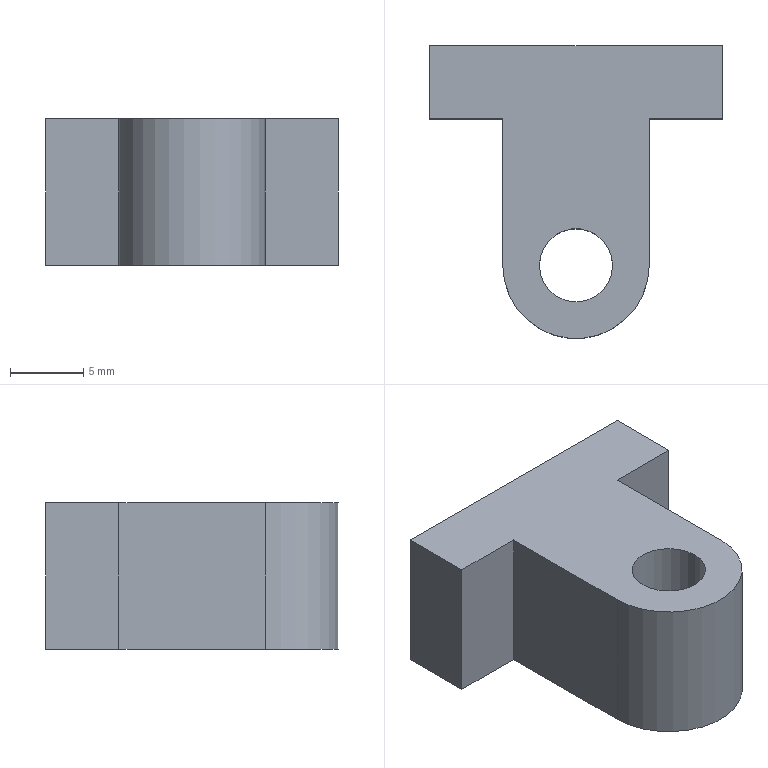Part | SolidWorks | features Extrusion 1, ICE 1 | 1 solid | 15 faces | box 20 x 20 x 10 mm | volume 2177 mm3 | plane 10 | cylinder 5 | commonest cylinder face diameters 5 x4 10 x1
STEP:
#1=CARTESIAN_POINT('',(0.,14.,2.5));
#2=VERTEX_POINT('',#1);
#3=CARTESIAN_POINT('',(0.,14.,7.5));
#4=VERTEX_POINT('',#3);
#5=CARTESIAN_POINT('',(0.,14.,5.));
#6=DIRECTION('',(0.,1.,0.));
#7=DIRECTION('',(0.,0.,1.));
#8=AXIS2_PLACEMENT_3D('',#5,#6,#7);
#9=CIRCLE('',#8,2.5);
#10=EDGE_CURVE('',#2,#4,#9,.T.);
#11=ORIENTED_EDGE('',*,*,#10,.F.);
#12=CARTESIAN_POINT('',(0.,15.,2.5));
#13=VERTEX_POINT('',#12);
#14=CARTESIAN_POINT('',(0.,14.,2.5));
#15=DIRECTION('',(0.,1.,0.));
#16=VECTOR('',#15,1000.);
#17=LINE('',#14,#16);
#18=EDGE_CURVE('',#2,#13,#17,.T.);
#19=ORIENTED_EDGE('',*,*,#18,.T.);
#20=CARTESIAN_POINT('',(0.,15.,7.5));
#21=VERTEX_POINT('',#20);
#22=CARTESIAN_POINT('',(0.,15.,5.));
#23=DIRECTION('',(0.,1.,0.));
#24=DIRECTION('',(0.,0.,1.));
#25=AXIS2_PLACEMENT_3D('',#22,#23,#24);
#26=CIRCLE('',#25,2.5);
#27=EDGE_CURVE('',#13,#21,#26,.T.);
#28=ORIENTED_EDGE('',*,*,#27,.T.);
#29=CARTESIAN_POINT('',(0.,14.,7.5));
#30=DIRECTION('',(0.,1.,0.));
#31=VECTOR('',#30,1000.);
#32=LINE('',#29,#31);
#33=EDGE_CURVE('',#4,#21,#32,.T.);
#34=ORIENTED_EDGE('',*,*,#33,.F.);
#35=EDGE_LOOP('',(#11,#19,#28,#34));
#36=FACE_OUTER_BOUND('',#35,.T.);
#37=CARTESIAN_POINT('',(0.,14.,5.));
#38=DIRECTION('',(0.,1.,0.));
#39=DIRECTION('',(0.,0.,1.));
#40=AXIS2_PLACEMENT_3D('',#37,#38,#39);
#41=CYLINDRICAL_SURFACE('',#40,2.5);
#42=ADVANCED_FACE('',(#36),#41,.F.);
#43=CARTESIAN_POINT('',(-2.5,0.,10.));
#44=VERTEX_POINT('',#43);
#45=CARTESIAN_POINT('',(2.5,0.,10.));
#46=VERTEX_POINT('',#45);
#47=CARTESIAN_POINT('',(0.,0.,10.));
#48=DIRECTION('',(0.,0.,1.));
#49=DIRECTION('',(1.,0.,0.));
#50=AXIS2_PLACEMENT_3D('',#47,#48,#49);
#51=CIRCLE('',#50,2.5);
#52=EDGE_CURVE('',#44,#46,#51,.T.);
#53=ORIENTED_EDGE('',*,*,#52,.T.);
#54=CARTESIAN_POINT('',(2.5,0.,0.));
#55=VERTEX_POINT('',#54);
#56=CARTESIAN_POINT('',(2.5,0.,10.));
#57=DIRECTION('',(0.,0.,-1.));
#58=VECTOR('',#57,1000.);
#59=LINE('',#56,#58);
#60=EDGE_CURVE('',#46,#55,#59,.T.);
#61=ORIENTED_EDGE('',*,*,#60,.T.);
#62=CARTESIAN_POINT('',(-2.5,0.,0.));
#63=VERTEX_POINT('',#62);
#64=CARTESIAN_POINT('',(0.,0.,0.));
#65=DIRECTION('',(0.,0.,1.));
#66=DIRECTION('',(1.,0.,0.));
#67=AXIS2_PLACEMENT_3D('',#64,#65,#66);
#68=CIRCLE('',#67,2.5);
#69=EDGE_CURVE('',#63,#55,#68,.T.);
#70=ORIENTED_EDGE('',*,*,#69,.F.);
#71=CARTESIAN_POINT('',(-2.5,0.,10.));
#72=DIRECTION('',(0.,0.,-1.));
#73=VECTOR('',#72,1000.);
#74=LINE('',#71,#73);
#75=EDGE_CURVE('',#44,#63,#74,.T.);
#76=ORIENTED_EDGE('',*,*,#75,.F.);
#77=EDGE_LOOP('',(#53,#61,#70,#76));
#78=FACE_OUTER_BOUND('',#77,.T.);
#79=CARTESIAN_POINT('',(0.,0.,10.));
#80=DIRECTION('',(0.,0.,-1.));
#81=DIRECTION('',(-1.,0.,0.));
#82=AXIS2_PLACEMENT_3D('',#79,#80,#81);
#83=CYLINDRICAL_SURFACE('',#82,2.5);
#84=ADVANCED_FACE('',(#78),#83,.F.);
#85=CARTESIAN_POINT('',(-5.,0.,10.));
#86=VERTEX_POINT('',#85);
#87=CARTESIAN_POINT('',(5.,0.,10.));
#88=VERTEX_POINT('',#87);
#89=CARTESIAN_POINT('',(0.,0.,10.));
#90=DIRECTION('',(0.,0.,1.));
#91=DIRECTION('',(1.,0.,0.));
#92=AXIS2_PLACEMENT_3D('',#89,#90,#91);
#93=CIRCLE('',#92,5.);
#94=EDGE_CURVE('',#86,#88,#93,.T.);
#95=ORIENTED_EDGE('',*,*,#94,.T.);
#96=CARTESIAN_POINT('',(5.,10.,10.));
#97=VERTEX_POINT('',#96);
#98=CARTESIAN_POINT('',(5.,0.,10.));
#99=DIRECTION('',(0.,1.,0.));
#100=VECTOR('',#99,1000.);
#101=LINE('',#98,#100);
#102=EDGE_CURVE('',#88,#97,#101,.T.);
#103=ORIENTED_EDGE('',*,*,#102,.T.);
#104=CARTESIAN_POINT('',(10.,10.,10.));
#105=VERTEX_POINT('',#104);
#106=CARTESIAN_POINT('',(5.,10.,10.));
#107=DIRECTION('',(1.,0.,0.));
#108=VECTOR('',#107,1000.);
#109=LINE('',#106,#108);
#110=EDGE_CURVE('',#97,#105,#109,.T.);
#111=ORIENTED_EDGE('',*,*,#110,.T.);
#112=CARTESIAN_POINT('',(10.,15.,10.));
#113=VERTEX_POINT('',#112);
#114=CARTESIAN_POINT('',(10.,10.,10.));
#115=DIRECTION('',(0.,1.,0.));
#116=VECTOR('',#115,1000.);
#117=LINE('',#114,#116);
#118=EDGE_CURVE('',#105,#113,#117,.T.);
#119=ORIENTED_EDGE('',*,*,#118,.T.);
#120=CARTESIAN_POINT('',(-10.,15.,10.));
#121=VERTEX_POINT('',#120);
#122=CARTESIAN_POINT('',(-10.,15.,10.));
#123=DIRECTION('',(-1.,0.,0.));
#124=VECTOR('',#123,1000.);
#125=LINE('',#122,#124);
#126=EDGE_CURVE('',#113,#121,#125,.T.);
#127=ORIENTED_EDGE('',*,*,#126,.T.);
#128=CARTESIAN_POINT('',(-10.,10.,10.));
#129=VERTEX_POINT('',#128);
#130=CARTESIAN_POINT('',(-10.,10.,10.));
#131=DIRECTION('',(0.,-1.,0.));
#132=VECTOR('',#131,1000.);
#133=LINE('',#130,#132);
#134=EDGE_CURVE('',#121,#129,#133,.T.);
#135=ORIENTED_EDGE('',*,*,#134,.T.);
#136=CARTESIAN_POINT('',(-5.,10.,10.));
#137=VERTEX_POINT('',#136);
#138=CARTESIAN_POINT('',(-5.,10.,10.));
#139=DIRECTION('',(1.,0.,0.));
#140=VECTOR('',#139,1000.);
#141=LINE('',#138,#140);
#142=EDGE_CURVE('',#129,#137,#141,.T.);
#143=ORIENTED_EDGE('',*,*,#142,.T.);
#144=CARTESIAN_POINT('',(-5.,0.,10.));
#145=DIRECTION('',(0.,-1.,0.));
#146=VECTOR('',#145,1000.);
#147=LINE('',#144,#146);
#148=EDGE_CURVE('',#137,#86,#147,.T.);
#149=ORIENTED_EDGE('',*,*,#148,.T.);
#150=EDGE_LOOP('',(#95,#103,#111,#119,#127,#135,#143,#149));
#151=FACE_OUTER_BOUND('',#150,.T.);
#152=ORIENTED_EDGE('',*,*,#52,.F.);
#153=CARTESIAN_POINT('',(0.,0.,10.));
#154=DIRECTION('',(0.,0.,1.));
#155=DIRECTION('',(1.,0.,0.));
#156=AXIS2_PLACEMENT_3D('',#153,#154,#155);
#157=CIRCLE('',#156,2.5);
#158=EDGE_CURVE('',#46,#44,#157,.T.);
#159=ORIENTED_EDGE('',*,*,#158,.F.);
#160=EDGE_LOOP('',(#152,#159));
#161=FACE_BOUND('',#160,.T.);
#162=CARTESIAN_POINT('',(0.,0.,10.));
#163=DIRECTION('',(0.,0.,1.));
#164=DIRECTION('',(1.,0.,0.));
#165=AXIS2_PLACEMENT_3D('',#162,#163,#164);
#166=PLANE('',#165);
#167=ADVANCED_FACE('',(#151,#161),#166,.T.);
#168=CARTESIAN_POINT('',(-5.,0.,0.));
#169=VERTEX_POINT('',#168);
#170=CARTESIAN_POINT('',(5.,0.,0.));
#171=VERTEX_POINT('',#170);
#172=CARTESIAN_POINT('',(0.,0.,0.));
#173=DIRECTION('',(0.,0.,1.));
#174=DIRECTION('',(1.,0.,0.));
#175=AXIS2_PLACEMENT_3D('',#172,#173,#174);
#176=CIRCLE('',#175,5.);
#177=EDGE_CURVE('',#169,#171,#176,.T.);
#178=ORIENTED_EDGE('',*,*,#177,.F.);
#179=CARTESIAN_POINT('',(-5.,10.,0.));
#180=VERTEX_POINT('',#179);
#181=CARTESIAN_POINT('',(-5.,0.,0.));
#182=DIRECTION('',(0.,-1.,0.));
#183=VECTOR('',#182,1000.);
#184=LINE('',#181,#183);
#185=EDGE_CURVE('',#180,#169,#184,.T.);
#186=ORIENTED_EDGE('',*,*,#185,.F.);
#187=CARTESIAN_POINT('',(-10.,10.,0.));
#188=VERTEX_POINT('',#187);
#189=CARTESIAN_POINT('',(-5.,10.,0.));
#190=DIRECTION('',(1.,0.,0.));
#191=VECTOR('',#190,1000.);
#192=LINE('',#189,#191);
#193=EDGE_CURVE('',#188,#180,#192,.T.);
#194=ORIENTED_EDGE('',*,*,#193,.F.);
#195=CARTESIAN_POINT('',(-10.,15.,0.));
#196=VERTEX_POINT('',#195);
#197=CARTESIAN_POINT('',(-10.,10.,0.));
#198=DIRECTION('',(0.,-1.,0.));
#199=VECTOR('',#198,1000.);
#200=LINE('',#197,#199);
#201=EDGE_CURVE('',#196,#188,#200,.T.);
#202=ORIENTED_EDGE('',*,*,#201,.F.);
#203=CARTESIAN_POINT('',(10.,15.,0.));
#204=VERTEX_POINT('',#203);
#205=CARTESIAN_POINT('',(-10.,15.,0.));
#206=DIRECTION('',(-1.,0.,0.));
#207=VECTOR('',#206,1000.);
#208=LINE('',#205,#207);
#209=EDGE_CURVE('',#204,#196,#208,.T.);
#210=ORIENTED_EDGE('',*,*,#209,.F.);
#211=CARTESIAN_POINT('',(10.,10.,0.));
#212=VERTEX_POINT('',#211);
#213=CARTESIAN_POINT('',(10.,10.,0.));
#214=DIRECTION('',(0.,1.,0.));
#215=VECTOR('',#214,1000.);
#216=LINE('',#213,#215);
#217=EDGE_CURVE('',#212,#204,#216,.T.);
#218=ORIENTED_EDGE('',*,*,#217,.F.);
#219=CARTESIAN_POINT('',(5.,10.,0.));
#220=VERTEX_POINT('',#219);
#221=CARTESIAN_POINT('',(5.,10.,0.));
#222=DIRECTION('',(1.,0.,0.));
#223=VECTOR('',#222,1000.);
#224=LINE('',#221,#223);
#225=EDGE_CURVE('',#220,#212,#224,.T.);
#226=ORIENTED_EDGE('',*,*,#225,.F.);
#227=CARTESIAN_POINT('',(5.,0.,0.));
#228=DIRECTION('',(0.,1.,0.));
#229=VECTOR('',#228,1000.);
#230=LINE('',#227,#229);
#231=EDGE_CURVE('',#171,#220,#230,.T.);
#232=ORIENTED_EDGE('',*,*,#231,.F.);
#233=EDGE_LOOP('',(#178,#186,#194,#202,#210,#218,#226,#232));
#234=FACE_OUTER_BOUND('',#233,.T.);
#235=ORIENTED_EDGE('',*,*,#69,.T.);
#236=CARTESIAN_POINT('',(0.,0.,0.));
#237=DIRECTION('',(0.,0.,1.));
#238=DIRECTION('',(1.,0.,0.));
#239=AXIS2_PLACEMENT_3D('',#236,#237,#238);
#240=CIRCLE('',#239,2.5);
#241=EDGE_CURVE('',#55,#63,#240,.T.);
#242=ORIENTED_EDGE('',*,*,#241,.T.);
#243=EDGE_LOOP('',(#235,#242));
#244=FACE_BOUND('',#243,.T.);
#245=CARTESIAN_POINT('',(0.,0.,0.));
#246=DIRECTION('',(0.,0.,1.));
#247=DIRECTION('',(1.,0.,0.));
#248=AXIS2_PLACEMENT_3D('',#245,#246,#247);
#249=PLANE('',#248);
#250=ADVANCED_FACE('',(#234,#244),#249,.F.);
#251=ORIENTED_EDGE('',*,*,#177,.T.);
#252=CARTESIAN_POINT('',(5.,0.,10.));
#253=DIRECTION('',(0.,0.,-1.));
#254=VECTOR('',#253,1000.);
#255=LINE('',#252,#254);
#256=EDGE_CURVE('',#88,#171,#255,.T.);
#257=ORIENTED_EDGE('',*,*,#256,.F.);
#258=ORIENTED_EDGE('',*,*,#94,.F.);
#259=CARTESIAN_POINT('',(-5.,0.,10.));
#260=DIRECTION('',(0.,0.,-1.));
#261=VECTOR('',#260,1000.);
#262=LINE('',#259,#261);
#263=EDGE_CURVE('',#86,#169,#262,.T.);
#264=ORIENTED_EDGE('',*,*,#263,.T.);
#265=EDGE_LOOP('',(#251,#257,#258,#264));
#266=FACE_OUTER_BOUND('',#265,.T.);
#267=CARTESIAN_POINT('',(0.,0.,10.));
#268=DIRECTION('',(0.,0.,-1.));
#269=DIRECTION('',(-1.,0.,0.));
#270=AXIS2_PLACEMENT_3D('',#267,#268,#269);
#271=CYLINDRICAL_SURFACE('',#270,5.);
#272=ADVANCED_FACE('',(#266),#271,.T.);
#273=ORIENTED_EDGE('',*,*,#231,.T.);
#274=CARTESIAN_POINT('',(5.,10.,10.));
#275=DIRECTION('',(0.,0.,-1.));
#276=VECTOR('',#275,1000.);
#277=LINE('',#274,#276);
#278=EDGE_CURVE('',#97,#220,#277,.T.);
#279=ORIENTED_EDGE('',*,*,#278,.F.);
#280=ORIENTED_EDGE('',*,*,#102,.F.);
#281=ORIENTED_EDGE('',*,*,#256,.T.);
#282=EDGE_LOOP('',(#273,#279,#280,#281));
#283=FACE_OUTER_BOUND('',#282,.T.);
#284=CARTESIAN_POINT('',(5.,0.,10.));
#285=DIRECTION('',(-1.,0.,0.));
#286=DIRECTION('',(0.,0.,1.));
#287=AXIS2_PLACEMENT_3D('',#284,#285,#286);
#288=PLANE('',#287);
#289=ADVANCED_FACE('',(#283),#288,.F.);
#290=ORIENTED_EDGE('',*,*,#225,.T.);
#291=CARTESIAN_POINT('',(10.,10.,10.));
#292=DIRECTION('',(0.,0.,-1.));
#293=VECTOR('',#292,1000.);
#294=LINE('',#291,#293);
#295=EDGE_CURVE('',#105,#212,#294,.T.);
#296=ORIENTED_EDGE('',*,*,#295,.F.);
#297=ORIENTED_EDGE('',*,*,#110,.F.);
#298=ORIENTED_EDGE('',*,*,#278,.T.);
#299=EDGE_LOOP('',(#290,#296,#297,#298));
#300=FACE_OUTER_BOUND('',#299,.T.);
#301=CARTESIAN_POINT('',(5.,10.,10.));
#302=DIRECTION('',(0.,1.,0.));
#303=DIRECTION('',(0.,0.,1.));
#304=AXIS2_PLACEMENT_3D('',#301,#302,#303);
#305=PLANE('',#304);
#306=ADVANCED_FACE('',(#300),#305,.F.);
#307=ORIENTED_EDGE('',*,*,#217,.T.);
#308=CARTESIAN_POINT('',(10.,15.,10.));
#309=DIRECTION('',(0.,0.,-1.));
#310=VECTOR('',#309,1000.);
#311=LINE('',#308,#310);
#312=EDGE_CURVE('',#113,#204,#311,.T.);
#313=ORIENTED_EDGE('',*,*,#312,.F.);
#314=ORIENTED_EDGE('',*,*,#118,.F.);
#315=ORIENTED_EDGE('',*,*,#295,.T.);
#316=EDGE_LOOP('',(#307,#313,#314,#315));
#317=FACE_OUTER_BOUND('',#316,.T.);
#318=CARTESIAN_POINT('',(10.,10.,10.));
#319=DIRECTION('',(-1.,0.,0.));
#320=DIRECTION('',(0.,0.,1.));
#321=AXIS2_PLACEMENT_3D('',#318,#319,#320);
#322=PLANE('',#321);
#323=ADVANCED_FACE('',(#317),#322,.F.);
#324=CARTESIAN_POINT('',(0.,15.,5.));
#325=DIRECTION('',(0.,1.,0.));
#326=DIRECTION('',(0.,0.,1.));
#327=AXIS2_PLACEMENT_3D('',#324,#325,#326);
#328=CIRCLE('',#327,2.5);
#329=EDGE_CURVE('',#21,#13,#328,.T.);
#330=ORIENTED_EDGE('',*,*,#329,.F.);
#331=ORIENTED_EDGE('',*,*,#27,.F.);
#332=EDGE_LOOP('',(#330,#331));
#333=FACE_BOUND('',#332,.T.);
#334=ORIENTED_EDGE('',*,*,#209,.T.);
#335=CARTESIAN_POINT('',(-10.,15.,10.));
#336=DIRECTION('',(0.,0.,-1.));
#337=VECTOR('',#336,1000.);
#338=LINE('',#335,#337);
#339=EDGE_CURVE('',#121,#196,#338,.T.);
#340=ORIENTED_EDGE('',*,*,#339,.F.);
#341=ORIENTED_EDGE('',*,*,#126,.F.);
#342=ORIENTED_EDGE('',*,*,#312,.T.);
#343=EDGE_LOOP('',(#334,#340,#341,#342));
#344=FACE_OUTER_BOUND('',#343,.T.);
#345=CARTESIAN_POINT('',(-10.,15.,10.));
#346=DIRECTION('',(0.,-1.,0.));
#347=DIRECTION('',(0.,0.,-1.));
#348=AXIS2_PLACEMENT_3D('',#345,#346,#347);
#349=PLANE('',#348);
#350=ADVANCED_FACE('',(#333,#344),#349,.F.);
#351=ORIENTED_EDGE('',*,*,#201,.T.);
#352=CARTESIAN_POINT('',(-10.,10.,10.));
#353=DIRECTION('',(0.,0.,-1.));
#354=VECTOR('',#353,1000.);
#355=LINE('',#352,#354);
#356=EDGE_CURVE('',#129,#188,#355,.T.);
#357=ORIENTED_EDGE('',*,*,#356,.F.);
#358=ORIENTED_EDGE('',*,*,#134,.F.);
#359=ORIENTED_EDGE('',*,*,#339,.T.);
#360=EDGE_LOOP('',(#351,#357,#358,#359));
#361=FACE_OUTER_BOUND('',#360,.T.);
#362=CARTESIAN_POINT('',(-10.,10.,10.));
#363=DIRECTION('',(1.,0.,0.));
#364=DIRECTION('',(0.,0.,-1.));
#365=AXIS2_PLACEMENT_3D('',#362,#363,#364);
#366=PLANE('',#365);
#367=ADVANCED_FACE('',(#361),#366,.F.);
#368=ORIENTED_EDGE('',*,*,#193,.T.);
#369=CARTESIAN_POINT('',(-5.,10.,10.));
#370=DIRECTION('',(0.,0.,-1.));
#371=VECTOR('',#370,1000.);
#372=LINE('',#369,#371);
#373=EDGE_CURVE('',#137,#180,#372,.T.);
#374=ORIENTED_EDGE('',*,*,#373,.F.);
#375=ORIENTED_EDGE('',*,*,#142,.F.);
#376=ORIENTED_EDGE('',*,*,#356,.T.);
#377=EDGE_LOOP('',(#368,#374,#375,#376));
#378=FACE_OUTER_BOUND('',#377,.T.);
#379=CARTESIAN_POINT('',(-5.,10.,10.));
#380=DIRECTION('',(0.,1.,0.));
#381=DIRECTION('',(0.,0.,1.));
#382=AXIS2_PLACEMENT_3D('',#379,#380,#381);
#383=PLANE('',#382);
#384=ADVANCED_FACE('',(#378),#383,.F.);
#385=ORIENTED_EDGE('',*,*,#185,.T.);
#386=ORIENTED_EDGE('',*,*,#263,.F.);
#387=ORIENTED_EDGE('',*,*,#148,.F.);
#388=ORIENTED_EDGE('',*,*,#373,.T.);
#389=EDGE_LOOP('',(#385,#386,#387,#388));
#390=FACE_OUTER_BOUND('',#389,.T.);
#391=CARTESIAN_POINT('',(-5.,0.,10.));
#392=DIRECTION('',(1.,0.,0.));
#393=DIRECTION('',(0.,0.,-1.));
#394=AXIS2_PLACEMENT_3D('',#391,#392,#393);
#395=PLANE('',#394);
#396=ADVANCED_FACE('',(#390),#395,.F.);
#397=ORIENTED_EDGE('',*,*,#60,.F.);
#398=ORIENTED_EDGE('',*,*,#158,.T.);
#399=ORIENTED_EDGE('',*,*,#75,.T.);
#400=ORIENTED_EDGE('',*,*,#241,.F.);
#401=EDGE_LOOP('',(#397,#398,#399,#400));
#402=FACE_OUTER_BOUND('',#401,.T.);
#403=CARTESIAN_POINT('',(0.,0.,10.));
#404=DIRECTION('',(0.,0.,-1.));
#405=DIRECTION('',(-1.,0.,0.));
#406=AXIS2_PLACEMENT_3D('',#403,#404,#405);
#407=CYLINDRICAL_SURFACE('',#406,2.5);
#408=ADVANCED_FACE('',(#402),#407,.F.);
#409=ORIENTED_EDGE('',*,*,#18,.F.);
#410=CARTESIAN_POINT('',(0.,14.,5.));
#411=DIRECTION('',(0.,1.,0.));
#412=DIRECTION('',(0.,0.,1.));
#413=AXIS2_PLACEMENT_3D('',#410,#411,#412);
#414=CIRCLE('',#413,2.5);
#415=EDGE_CURVE('',#4,#2,#414,.T.);
#416=ORIENTED_EDGE('',*,*,#415,.F.);
#417=ORIENTED_EDGE('',*,*,#33,.T.);
#418=ORIENTED_EDGE('',*,*,#329,.T.);
#419=EDGE_LOOP('',(#409,#416,#417,#418));
#420=FACE_OUTER_BOUND('',#419,.T.);
#421=CARTESIAN_POINT('',(0.,14.,5.));
#422=DIRECTION('',(0.,1.,0.));
#423=DIRECTION('',(0.,0.,1.));
#424=AXIS2_PLACEMENT_3D('',#421,#422,#423);
#425=CYLINDRICAL_SURFACE('',#424,2.5);
#426=ADVANCED_FACE('',(#420),#425,.F.);
#427=ORIENTED_EDGE('',*,*,#415,.T.);
#428=ORIENTED_EDGE('',*,*,#10,.T.);
#429=EDGE_LOOP('',(#427,#428));
#430=FACE_OUTER_BOUND('',#429,.T.);
#431=CARTESIAN_POINT('',(0.,14.,5.));
#432=DIRECTION('',(0.,1.,0.));
#433=DIRECTION('',(0.,0.,1.));
#434=AXIS2_PLACEMENT_3D('',#431,#432,#433);
#435=PLANE('',#434);
#436=ADVANCED_FACE('',(#430),#435,.T.);
#437=CLOSED_SHELL('',(#42,#84,#167,#250,#272,#289,#306,#323,#350,#367,#384,#396,#408,#426,#436));
#438=MANIFOLD_SOLID_BREP('',#437);
#439=CARTESIAN_POINT('',(0.,0.,0.));
#440=DIRECTION('',(0.,0.,1.));
#441=DIRECTION('',(1.,0.,0.));
#442=AXIS2_PLACEMENT_3D('',#439,#440,#441);
#443=(LENGTH_UNIT()NAMED_UNIT(*)SI_UNIT(.MILLI.,.METRE.));
#444=UNCERTAINTY_MEASURE_WITH_UNIT(LENGTH_MEASURE(0.00001),#443,'','');
#445=(NAMED_UNIT(*)PLANE_ANGLE_UNIT()SI_UNIT($,.RADIAN.));
#446=(NAMED_UNIT(*)SI_UNIT($,.STERADIAN.)SOLID_ANGLE_UNIT());
#447=(GEOMETRIC_REPRESENTATION_CONTEXT(3)GLOBAL_UNCERTAINTY_ASSIGNED_CONTEXT((#444))GLOBAL_UNIT_ASSIGNED_CONTEXT((#443,#445,#446))REPRESENTATION_CONTEXT('',''));
#448=ADVANCED_BREP_SHAPE_REPRESENTATION('',(#438,#442),#447);